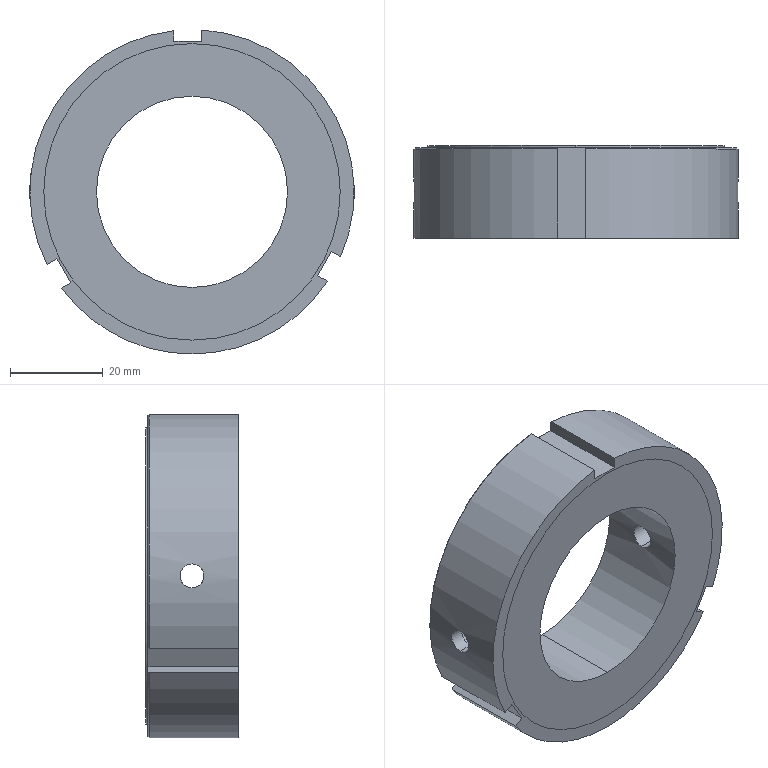Part | STEP file | 2 solids | 35 faces | box 70 x 20 x 69.938 mm | volume 48420 mm3 | cylinder 18 | plane 13 | cone 4 | commonest cylinder face diameters 5.16 x8 64 x4 70 x4 41.28 x2